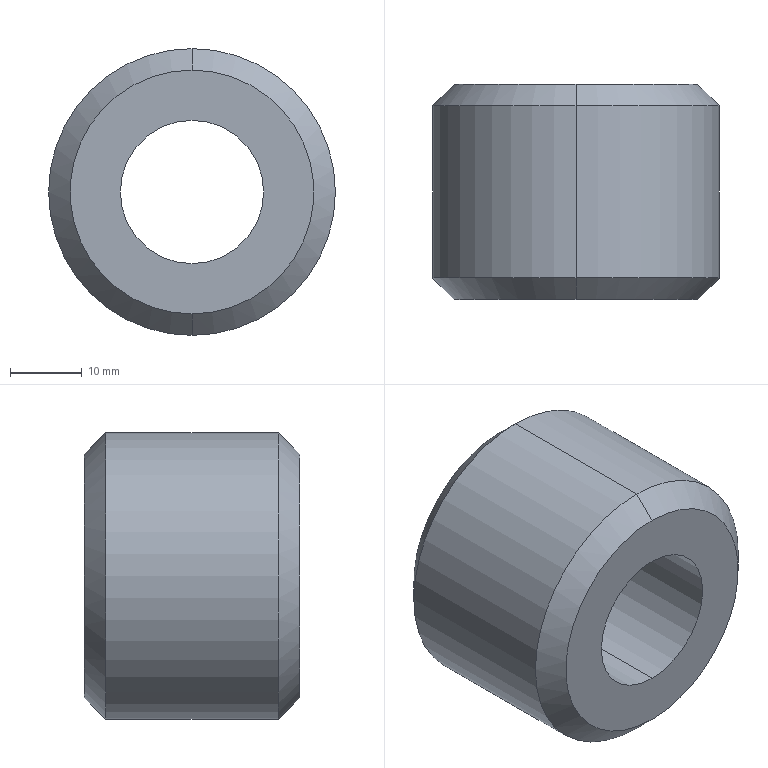Part | SolidWorks | features Chamfer 1, Extrusion 1 | 1 solid | 10 faces | box 40 x 30 x 40 mm | volume 27200 mm3 | cone 4 | cylinder 4 | plane 2 | commonest cylinder face diameters 20 x2 40 x2
STEP:
#1=CARTESIAN_POINT('',(0.,30.,17.));
#2=VERTEX_POINT('',#1);
#3=CARTESIAN_POINT('',(0.,30.,-17.));
#4=VERTEX_POINT('',#3);
#5=CARTESIAN_POINT('',(0.,30.,0.));
#6=DIRECTION('',(0.,1.,0.));
#7=DIRECTION('',(0.,0.,1.));
#8=AXIS2_PLACEMENT_3D('',#5,#6,#7);
#9=CIRCLE('',#8,17.);
#10=EDGE_CURVE('',#2,#4,#9,.T.);
#11=ORIENTED_EDGE('',*,*,#10,.F.);
#12=CARTESIAN_POINT('',(0.,27.,20.));
#13=VERTEX_POINT('',#12);
#14=CARTESIAN_POINT('',(0.,30.,17.));
#15=DIRECTION('',(0.,-0.7071,0.7071));
#16=VECTOR('',#15,1000.);
#17=LINE('',#14,#16);
#18=EDGE_CURVE('',#2,#13,#17,.T.);
#19=ORIENTED_EDGE('',*,*,#18,.T.);
#20=CARTESIAN_POINT('',(0.,27.,-20.));
#21=VERTEX_POINT('',#20);
#22=CARTESIAN_POINT('',(0.,27.,0.));
#23=DIRECTION('',(0.,-1.,0.));
#24=DIRECTION('',(0.,0.,1.));
#25=AXIS2_PLACEMENT_3D('',#22,#23,#24);
#26=CIRCLE('',#25,20.);
#27=EDGE_CURVE('',#21,#13,#26,.T.);
#28=ORIENTED_EDGE('',*,*,#27,.F.);
#29=CARTESIAN_POINT('',(0.,30.,-17.));
#30=DIRECTION('',(0.,-0.7071,-0.7071));
#31=VECTOR('',#30,1000.);
#32=LINE('',#29,#31);
#33=EDGE_CURVE('',#4,#21,#32,.T.);
#34=ORIENTED_EDGE('',*,*,#33,.F.);
#35=EDGE_LOOP('',(#11,#19,#28,#34));
#36=FACE_OUTER_BOUND('',#35,.T.);
#37=CARTESIAN_POINT('',(0.,30.,0.));
#38=DIRECTION('',(0.,-1.,0.));
#39=DIRECTION('',(0.,0.,-1.));
#40=AXIS2_PLACEMENT_3D('',#37,#38,#39);
#41=CONICAL_SURFACE('',#40,17.,0.7854);
#42=ADVANCED_FACE('',(#36),#41,.T.);
#43=CARTESIAN_POINT('',(0.,0.,-17.));
#44=VERTEX_POINT('',#43);
#45=CARTESIAN_POINT('',(0.,0.,17.));
#46=VERTEX_POINT('',#45);
#47=CARTESIAN_POINT('',(0.,0.,0.));
#48=DIRECTION('',(0.,-1.,0.));
#49=DIRECTION('',(0.,0.,1.));
#50=AXIS2_PLACEMENT_3D('',#47,#48,#49);
#51=CIRCLE('',#50,17.);
#52=EDGE_CURVE('',#44,#46,#51,.T.);
#53=ORIENTED_EDGE('',*,*,#52,.F.);
#54=CARTESIAN_POINT('',(0.,3.,-20.));
#55=VERTEX_POINT('',#54);
#56=CARTESIAN_POINT('',(0.,3.,-20.));
#57=DIRECTION('',(0.,0.7071,-0.7071));
#58=VECTOR('',#57,1000.);
#59=LINE('',#56,#58);
#60=EDGE_CURVE('',#44,#55,#59,.T.);
#61=ORIENTED_EDGE('',*,*,#60,.T.);
#62=CARTESIAN_POINT('',(0.,3.,20.));
#63=VERTEX_POINT('',#62);
#64=CARTESIAN_POINT('',(0.,3.,0.));
#65=DIRECTION('',(0.,1.,0.));
#66=DIRECTION('',(0.,0.,1.));
#67=AXIS2_PLACEMENT_3D('',#64,#65,#66);
#68=CIRCLE('',#67,20.);
#69=EDGE_CURVE('',#63,#55,#68,.T.);
#70=ORIENTED_EDGE('',*,*,#69,.F.);
#71=CARTESIAN_POINT('',(0.,3.,20.));
#72=DIRECTION('',(0.,0.7071,0.7071));
#73=VECTOR('',#72,1000.);
#74=LINE('',#71,#73);
#75=EDGE_CURVE('',#46,#63,#74,.T.);
#76=ORIENTED_EDGE('',*,*,#75,.F.);
#77=EDGE_LOOP('',(#53,#61,#70,#76));
#78=FACE_OUTER_BOUND('',#77,.T.);
#79=CARTESIAN_POINT('',(0.,3.,0.));
#80=DIRECTION('',(0.,1.,0.));
#81=DIRECTION('',(0.,0.,1.));
#82=AXIS2_PLACEMENT_3D('',#79,#80,#81);
#83=CONICAL_SURFACE('',#82,20.,0.7854);
#84=ADVANCED_FACE('',(#78),#83,.T.);
#85=CARTESIAN_POINT('',(0.,30.,-10.));
#86=VERTEX_POINT('',#85);
#87=CARTESIAN_POINT('',(0.,30.,10.));
#88=VERTEX_POINT('',#87);
#89=CARTESIAN_POINT('',(0.,30.,0.));
#90=DIRECTION('',(0.,1.,0.));
#91=DIRECTION('',(0.,0.,1.));
#92=AXIS2_PLACEMENT_3D('',#89,#90,#91);
#93=CIRCLE('',#92,10.);
#94=EDGE_CURVE('',#86,#88,#93,.T.);
#95=ORIENTED_EDGE('',*,*,#94,.T.);
#96=CARTESIAN_POINT('',(0.,0.,10.));
#97=VERTEX_POINT('',#96);
#98=CARTESIAN_POINT('',(0.,30.,10.));
#99=DIRECTION('',(0.,-1.,0.));
#100=VECTOR('',#99,1000.);
#101=LINE('',#98,#100);
#102=EDGE_CURVE('',#88,#97,#101,.T.);
#103=ORIENTED_EDGE('',*,*,#102,.T.);
#104=CARTESIAN_POINT('',(0.,0.,-10.));
#105=VERTEX_POINT('',#104);
#106=CARTESIAN_POINT('',(0.,0.,0.));
#107=DIRECTION('',(0.,1.,0.));
#108=DIRECTION('',(0.,0.,1.));
#109=AXIS2_PLACEMENT_3D('',#106,#107,#108);
#110=CIRCLE('',#109,10.);
#111=EDGE_CURVE('',#105,#97,#110,.T.);
#112=ORIENTED_EDGE('',*,*,#111,.F.);
#113=CARTESIAN_POINT('',(0.,30.,-10.));
#114=DIRECTION('',(0.,-1.,0.));
#115=VECTOR('',#114,1000.);
#116=LINE('',#113,#115);
#117=EDGE_CURVE('',#86,#105,#116,.T.);
#118=ORIENTED_EDGE('',*,*,#117,.F.);
#119=EDGE_LOOP('',(#95,#103,#112,#118));
#120=FACE_OUTER_BOUND('',#119,.T.);
#121=CARTESIAN_POINT('',(0.,30.,0.));
#122=DIRECTION('',(0.,-1.,0.));
#123=DIRECTION('',(0.,0.,-1.));
#124=AXIS2_PLACEMENT_3D('',#121,#122,#123);
#125=CYLINDRICAL_SURFACE('',#124,10.);
#126=ADVANCED_FACE('',(#120),#125,.F.);
#127=ORIENTED_EDGE('',*,*,#27,.T.);
#128=CARTESIAN_POINT('',(0.,30.,20.));
#129=DIRECTION('',(0.,-1.,0.));
#130=VECTOR('',#129,1000.);
#131=LINE('',#128,#130);
#132=EDGE_CURVE('',#13,#63,#131,.T.);
#133=ORIENTED_EDGE('',*,*,#132,.T.);
#134=ORIENTED_EDGE('',*,*,#69,.T.);
#135=CARTESIAN_POINT('',(0.,30.,-20.));
#136=DIRECTION('',(0.,-1.,0.));
#137=VECTOR('',#136,1000.);
#138=LINE('',#135,#137);
#139=EDGE_CURVE('',#21,#55,#138,.T.);
#140=ORIENTED_EDGE('',*,*,#139,.F.);
#141=EDGE_LOOP('',(#127,#133,#134,#140));
#142=FACE_OUTER_BOUND('',#141,.T.);
#143=CARTESIAN_POINT('',(0.,30.,0.));
#144=DIRECTION('',(0.,-1.,0.));
#145=DIRECTION('',(0.,0.,-1.));
#146=AXIS2_PLACEMENT_3D('',#143,#144,#145);
#147=CYLINDRICAL_SURFACE('',#146,20.);
#148=ADVANCED_FACE('',(#142),#147,.T.);
#149=CARTESIAN_POINT('',(0.,30.,0.));
#150=DIRECTION('',(0.,1.,0.));
#151=DIRECTION('',(0.,0.,1.));
#152=AXIS2_PLACEMENT_3D('',#149,#150,#151);
#153=CIRCLE('',#152,17.);
#154=EDGE_CURVE('',#4,#2,#153,.T.);
#155=ORIENTED_EDGE('',*,*,#154,.T.);
#156=ORIENTED_EDGE('',*,*,#10,.T.);
#157=EDGE_LOOP('',(#155,#156));
#158=FACE_OUTER_BOUND('',#157,.T.);
#159=ORIENTED_EDGE('',*,*,#94,.F.);
#160=CARTESIAN_POINT('',(0.,30.,0.));
#161=DIRECTION('',(0.,1.,0.));
#162=DIRECTION('',(0.,0.,1.));
#163=AXIS2_PLACEMENT_3D('',#160,#161,#162);
#164=CIRCLE('',#163,10.);
#165=EDGE_CURVE('',#88,#86,#164,.T.);
#166=ORIENTED_EDGE('',*,*,#165,.F.);
#167=EDGE_LOOP('',(#159,#166));
#168=FACE_BOUND('',#167,.T.);
#169=CARTESIAN_POINT('',(0.,30.,0.));
#170=DIRECTION('',(0.,1.,0.));
#171=DIRECTION('',(0.,0.,1.));
#172=AXIS2_PLACEMENT_3D('',#169,#170,#171);
#173=PLANE('',#172);
#174=ADVANCED_FACE('',(#158,#168),#173,.T.);
#175=CARTESIAN_POINT('',(0.,0.,0.));
#176=DIRECTION('',(0.,-1.,0.));
#177=DIRECTION('',(0.,0.,1.));
#178=AXIS2_PLACEMENT_3D('',#175,#176,#177);
#179=CIRCLE('',#178,17.);
#180=EDGE_CURVE('',#46,#44,#179,.T.);
#181=ORIENTED_EDGE('',*,*,#180,.T.);
#182=ORIENTED_EDGE('',*,*,#52,.T.);
#183=EDGE_LOOP('',(#181,#182));
#184=FACE_OUTER_BOUND('',#183,.T.);
#185=ORIENTED_EDGE('',*,*,#111,.T.);
#186=CARTESIAN_POINT('',(0.,0.,0.));
#187=DIRECTION('',(0.,1.,0.));
#188=DIRECTION('',(0.,0.,1.));
#189=AXIS2_PLACEMENT_3D('',#186,#187,#188);
#190=CIRCLE('',#189,10.);
#191=EDGE_CURVE('',#97,#105,#190,.T.);
#192=ORIENTED_EDGE('',*,*,#191,.T.);
#193=EDGE_LOOP('',(#185,#192));
#194=FACE_BOUND('',#193,.T.);
#195=CARTESIAN_POINT('',(0.,0.,0.));
#196=DIRECTION('',(0.,1.,0.));
#197=DIRECTION('',(0.,0.,1.));
#198=AXIS2_PLACEMENT_3D('',#195,#196,#197);
#199=PLANE('',#198);
#200=ADVANCED_FACE('',(#184,#194),#199,.F.);
#201=ORIENTED_EDGE('',*,*,#132,.F.);
#202=CARTESIAN_POINT('',(0.,27.,0.));
#203=DIRECTION('',(0.,-1.,0.));
#204=DIRECTION('',(0.,0.,1.));
#205=AXIS2_PLACEMENT_3D('',#202,#203,#204);
#206=CIRCLE('',#205,20.);
#207=EDGE_CURVE('',#13,#21,#206,.T.);
#208=ORIENTED_EDGE('',*,*,#207,.T.);
#209=ORIENTED_EDGE('',*,*,#139,.T.);
#210=CARTESIAN_POINT('',(0.,3.,0.));
#211=DIRECTION('',(0.,1.,0.));
#212=DIRECTION('',(0.,0.,1.));
#213=AXIS2_PLACEMENT_3D('',#210,#211,#212);
#214=CIRCLE('',#213,20.);
#215=EDGE_CURVE('',#55,#63,#214,.T.);
#216=ORIENTED_EDGE('',*,*,#215,.T.);
#217=EDGE_LOOP('',(#201,#208,#209,#216));
#218=FACE_OUTER_BOUND('',#217,.T.);
#219=CARTESIAN_POINT('',(0.,30.,0.));
#220=DIRECTION('',(0.,-1.,0.));
#221=DIRECTION('',(0.,0.,-1.));
#222=AXIS2_PLACEMENT_3D('',#219,#220,#221);
#223=CYLINDRICAL_SURFACE('',#222,20.);
#224=ADVANCED_FACE('',(#218),#223,.T.);
#225=ORIENTED_EDGE('',*,*,#102,.F.);
#226=ORIENTED_EDGE('',*,*,#165,.T.);
#227=ORIENTED_EDGE('',*,*,#117,.T.);
#228=ORIENTED_EDGE('',*,*,#191,.F.);
#229=EDGE_LOOP('',(#225,#226,#227,#228));
#230=FACE_OUTER_BOUND('',#229,.T.);
#231=CARTESIAN_POINT('',(0.,30.,0.));
#232=DIRECTION('',(0.,-1.,0.));
#233=DIRECTION('',(0.,0.,-1.));
#234=AXIS2_PLACEMENT_3D('',#231,#232,#233);
#235=CYLINDRICAL_SURFACE('',#234,10.);
#236=ADVANCED_FACE('',(#230),#235,.F.);
#237=ORIENTED_EDGE('',*,*,#60,.F.);
#238=ORIENTED_EDGE('',*,*,#180,.F.);
#239=ORIENTED_EDGE('',*,*,#75,.T.);
#240=ORIENTED_EDGE('',*,*,#215,.F.);
#241=EDGE_LOOP('',(#237,#238,#239,#240));
#242=FACE_OUTER_BOUND('',#241,.T.);
#243=CARTESIAN_POINT('',(0.,3.,0.));
#244=DIRECTION('',(0.,1.,0.));
#245=DIRECTION('',(0.,0.,1.));
#246=AXIS2_PLACEMENT_3D('',#243,#244,#245);
#247=CONICAL_SURFACE('',#246,20.,0.7854);
#248=ADVANCED_FACE('',(#242),#247,.T.);
#249=ORIENTED_EDGE('',*,*,#18,.F.);
#250=ORIENTED_EDGE('',*,*,#154,.F.);
#251=ORIENTED_EDGE('',*,*,#33,.T.);
#252=ORIENTED_EDGE('',*,*,#207,.F.);
#253=EDGE_LOOP('',(#249,#250,#251,#252));
#254=FACE_OUTER_BOUND('',#253,.T.);
#255=CARTESIAN_POINT('',(0.,30.,0.));
#256=DIRECTION('',(0.,-1.,0.));
#257=DIRECTION('',(0.,0.,-1.));
#258=AXIS2_PLACEMENT_3D('',#255,#256,#257);
#259=CONICAL_SURFACE('',#258,17.,0.7854);
#260=ADVANCED_FACE('',(#254),#259,.T.);
#261=CLOSED_SHELL('',(#42,#84,#126,#148,#174,#200,#224,#236,#248,#260));
#262=MANIFOLD_SOLID_BREP('',#261);
#263=CARTESIAN_POINT('',(0.,0.,0.));
#264=DIRECTION('',(0.,0.,1.));
#265=DIRECTION('',(1.,0.,0.));
#266=AXIS2_PLACEMENT_3D('',#263,#264,#265);
#267=(LENGTH_UNIT()NAMED_UNIT(*)SI_UNIT(.MILLI.,.METRE.));
#268=UNCERTAINTY_MEASURE_WITH_UNIT(LENGTH_MEASURE(0.00001),#267,'','');
#269=(NAMED_UNIT(*)PLANE_ANGLE_UNIT()SI_UNIT($,.RADIAN.));
#270=(NAMED_UNIT(*)SI_UNIT($,.STERADIAN.)SOLID_ANGLE_UNIT());
#271=(GEOMETRIC_REPRESENTATION_CONTEXT(3)GLOBAL_UNCERTAINTY_ASSIGNED_CONTEXT((#268))GLOBAL_UNIT_ASSIGNED_CONTEXT((#267,#269,#270))REPRESENTATION_CONTEXT('',''));
#272=ADVANCED_BREP_SHAPE_REPRESENTATION('',(#262,#266),#271);